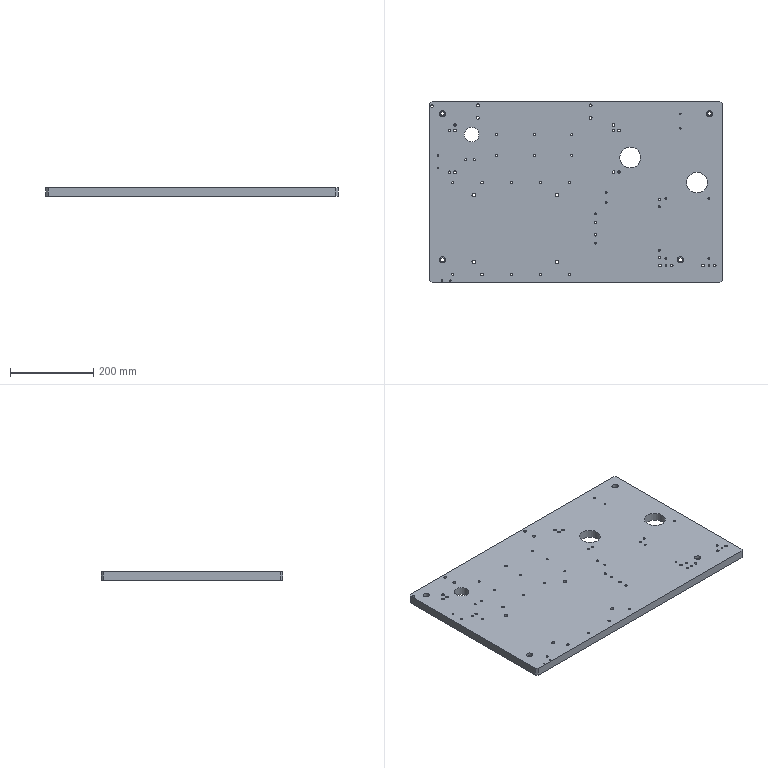CAM job | NX | 3-axis milling, drilling | part box 700 x 435 x 20 mm | stock box 700 x 435 x 20 mm
Tools:
number,name,description,diameter,corner_radius,flute_length,length,flutes
6,D6,平底铣刀-粗,6.0,0.0,25.0,75.0,2
9,D10,平底铣刀-粗,10.0,0.0,35.0,75.0,2
7,D6-J,平底铣刀-精,6.0,0.0,25.0,75.0,2
10,D10-J,平底铣刀-精,10.0,0.0,35.0,75.0,2
2,D6倒角刀,倒角刀,6.0,0.0,3.0,25.0,2
21,M4X0.7,丝锥,3.3,0.0,35.0,50.0,2
22,M5X0.8,丝锥,4.2,0.0,35.0,50.0,2
23,M6X1.0,丝锥,5.0,0.0,35.0,50.0,2
24,M8X1.25,丝锥,6.8,0.0,35.0,50.0,2
19,M10X1.5,丝锥,8.5,0.0,35.0,50.0,2
11,D6铰刀,Drilling Tool,6.0,0.0,75.0,100.0,6
1,C6定点钻,倒角刀,6.0,0.0,3.0,3.0,2
13,ZT3.4,钻头,3.4,0.0,35.0,50.0,2
15,ZT5.1,钻头,5.1,0.0,35.0,50.0,2
17,ZT8.7,钻头,8.7,0.0,35.0,50.0,2
20,ZT9,钻头,9.0,0.0,35.0,50.0,2
18,ZT5.9,Drilling Tool,5.9,0.0,35.0,50.0,2
16,ZT6.9,Drilling Tool,6.9,0.0,35.0,50.0,2
14,ZT4.3,Drilling Tool,4.3,0.0,50.0,75.0,4
Operations:
program,operation,operation_type,tool,method,geometry_group,spindle_rpm,surface_speed,feed_per_tooth,feed_cut,feed_plunge,cut_length_mm,path_length_mm,cut_time_min,machine_time_min
B,MILLCHAMFER_6,PlanarMilling,D6倒角刀,METHOD,W-B,4000.0,75.398,0.0375,300.0,100.0,360.407,4217.58,1.201,1.587
B,MILLCHAMFER_7,PlanarMilling,D6倒角刀,METHOD,W-B,4000.0,75.398,0.075,600.0,100.0,378.427,4398.443,0.6307,1.033
B,MILLCHAMFER_8,PlanarMilling,D6倒角刀,METHOD,W-B,4000.0,75.398,0.0375,300.0,100.0,191.323,1664.35,0.6377,0.785
B,MILLCHAMFER_9,PlanarMilling,D6倒角刀,METHOD,W-B,3000.0,56.549,0.0667,400.0,100.0,140.605,1068.68,0.3515,0.4443
B,MILLCHAMFER_10,PlanarMilling,D6倒角刀,METHOD,W-B,3000.0,56.549,0.1,600.0,100.0,93.674,1785.072,0.1561,0.3253
B,PLANARDEBURR_6X45L_COPY_1,SurfaceContour,D6倒角刀,CLIMBCHAMFER-DEPTH0-STEPG,W-B,3500.0,65.972,0.1429,1000.0,100.0,2796.64,12071.274,2.797,3.724
A,LINEZIGZAGLAYER_ROUGH-MID_COPY,PlanarMilling,D10,LAYERROUGH-DEPTHK-STEPG,W-A,3000.0,94.245,0.3333,2000.0,100.0,5716.203,7798.857,2.858,3.066
A,SPOTDRILL-DEPTH0.8,Operation,C6定点钻,NONE,W-A,3000.0,56.0,0.01,60.0,90.0,126.0,3815.301,2.1,2.469
A,THROUGH-M6_TAPDRILL,Operation,ZT5.1,NONE,W-A,800.0,12.566,0.0625,100.0,90.0,540.0,2989.198,5.4,5.645
A,THROUGH-FINISH6.0_PREDRILL,Operation,ZT5.9,NONE,W-A,1000.0,18.535,0.04,80.0,90.0,539.767,3018.349,6.747,6.995
A,THROUGH-M8_TAPDRILL,Operation,ZT6.9,NONE,W-A,600.0,12.818,0.1,120.0,90.0,232.0,1226.361,1.933,2.033
A,THROUGH-M10_TAPDRILL,Operation,ZT8.7,NONE,W-A,500.0,13.352,0.12,120.0,90.0,120.0,863.009,1.0,1.074
A,COUNTERSINK-DRILL_SEG0,Operation,ZT9,NONE,W-A,500.0,14.137,0.12,120.0,90.0,102.816,1585.566,0.8568,1.005
A,BLINDCONE-M4_TAPDRILL,Operation,ZT3.4,NONE,W-A,1500.0,15.551,0.02,60.0,90.0,75.0,1193.84,1.25,1.362
A,BLINDCONE-M5_TAPDRILL,Operation,ZT4.3,NONE,W-A,1200.0,15.834,0.0333,80.0,90.0,60.0,469.875,0.75,0.791
A,BOTTOMWALL_HELIXROUGH-MID_COPY,VolumeBased25DMillingOperation,D10,LAYERROUGH-DEPTHK-STEPG,W-A,3000.0,94.245,0.3333,2000.0,100.0,33282.978,34183.829,16.642,16.732
A,HOLEMILL_ROUGH_D8_1,CylinderMilling,D6,NONE,W-A,4000.0,75.398,0.1875,1500.0,100.0,6287.198,8102.929,4.191,4.373
A,HOLEMILL_FINISH_D8_1,CylinderMilling,D6-J,FINISHSTEPDEPTHOFF,W-A,4000.0,100.531,0.1,800.0,100.0,374.596,2153.927,0.4682,0.6462
A,BOTTOMWALL_FINISHSIDE-MID_COPY,VolumeBased25DMillingOperation,D6-J,SIDEFINISH-DEPTHK-STEPG,W-A,3500.0,65.972,0.1143,800.0,100.0,1162.755,1920.014,1.453,1.529
A,DRILLCHAMFER_1,Operation,D6倒角刀,METHOD,W-A,4000.0,75.398,0.01,80.0,0.0,31.2,1116.707,0.39,0.4986
A,MILLCHAMFER_1,PlanarMilling,D6倒角刀,METHOD,W-A,4000.0,75.398,0.0375,300.0,100.0,72.081,725.606,0.2403,0.3056
A,MILLCHAMFER_2,PlanarMilling,D6倒角刀,METHOD,W-A,4000.0,75.398,0.0375,300.0,100.0,398.764,4237.963,1.329,1.713
A,MILLCHAMFER_3,PlanarMilling,D6倒角刀,METHOD,W-A,4000.0,75.398,0.05,400.0,100.0,440.238,4427.365,1.101,1.499
A,MILLCHAMFER_4,PlanarMilling,D6倒角刀,METHOD,W-A,4000.0,75.398,0.0625,500.0,100.0,187.816,1659.243,0.3756,0.5228
A,MILLCHAMFER_5,PlanarMilling,D6倒角刀,METHOD,W-A,4000.0,75.398,0.0625,500.0,100.0,137.735,1065.804,0.2755,0.3683
A,PLANARDEBURR_6X45L_COPY,SurfaceContour,D6倒角刀,CLIMBCHAMFER-DEPTH0-STEPG,W-A,3500.0,65.972,0.1429,1000.0,100.0,3118.365,17296.075,3.118,4.536
A,REAMING,Operation,D6铰刀,METHOD,W-A,500.0,9.425,0.0167,50.0,0.0,462.0,2862.815,9.24,9.48
A,THROUGH-TAPM6,Operation,M6X1.0,METHOD,W-A,400.0,6.283,0.0013,1.0,90.0,490.0,2889.198,490.0,490.24
A,THROUGH-TAPM8,Operation,M8X1.25,METHOD,W-A,300.0,6.409,0.0021,1.25,90.0,204.0,1170.361,163.2,163.297
A,THROUGH-TAPM10,Operation,M10X1.5,METHOD,W-A,200.0,5.341,0.0037,1.5,90.0,104.0,831.009,69.333,69.406
A,BLINDCONE-TAPM4,Operation,M4X0.7,METHOD,W-A,600.0,6.22,0.0006,0.7,90.0,54.6,1153.04,78.0,78.11
A,BLINDCONE-TAPM5,Operation,M5X0.8,METHOD,W-A,500.0,6.597,0.0008,0.8,90.0,43.6,437.075,54.5,54.539
A,PLANARMILL_FINISHSIDE-MID-LINE_COPY,PlanarMilling,D10-J,SIDEFINISH-DEPTHK-STEPG,W-A,3000.0,94.245,0.1333,800.0,100.0,252.853,3469.179,0.3161,0.6377